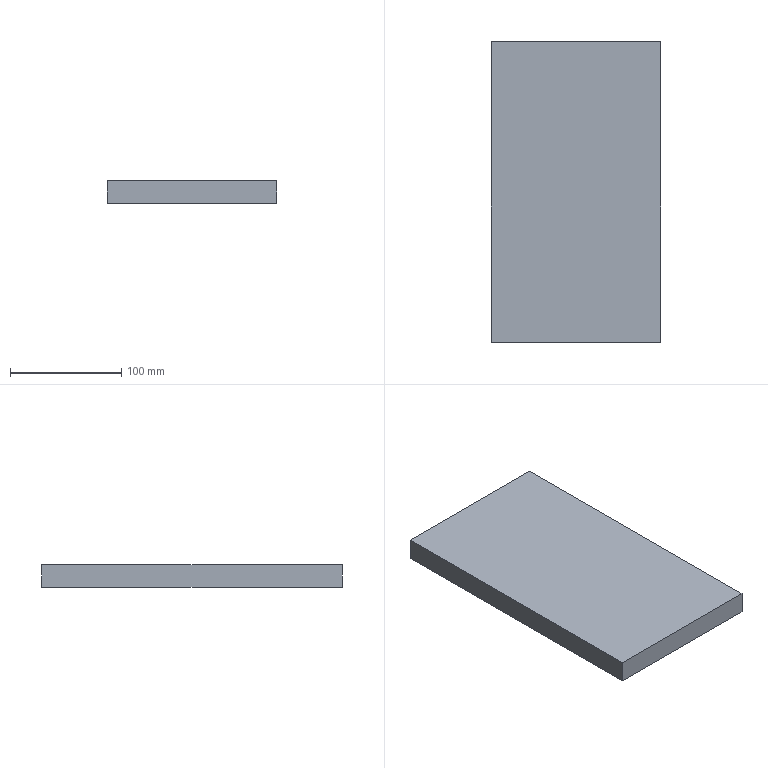Part | SolidWorks | features Extrusion 1 | 1 solid | 6 faces | box 152 x 270 x 20 mm | volume 820800 mm3 | plane 6
STEP:
#1=CARTESIAN_POINT('',(0.,270.,0.));
#2=VERTEX_POINT('',#1);
#3=CARTESIAN_POINT('',(0.,0.,0.));
#4=VERTEX_POINT('',#3);
#5=CARTESIAN_POINT('',(0.,0.,0.));
#6=DIRECTION('',(0.,-1.,0.));
#7=VECTOR('',#6,1000.);
#8=LINE('',#5,#7);
#9=EDGE_CURVE('',#2,#4,#8,.T.);
#10=ORIENTED_EDGE('',*,*,#9,.T.);
#11=CARTESIAN_POINT('',(0.,0.,20.));
#12=VERTEX_POINT('',#11);
#13=CARTESIAN_POINT('',(0.,0.,20.));
#14=DIRECTION('',(0.,0.,-1.));
#15=VECTOR('',#14,1000.);
#16=LINE('',#13,#15);
#17=EDGE_CURVE('',#12,#4,#16,.T.);
#18=ORIENTED_EDGE('',*,*,#17,.F.);
#19=CARTESIAN_POINT('',(0.,270.,20.));
#20=VERTEX_POINT('',#19);
#21=CARTESIAN_POINT('',(0.,0.,20.));
#22=DIRECTION('',(0.,-1.,0.));
#23=VECTOR('',#22,1000.);
#24=LINE('',#21,#23);
#25=EDGE_CURVE('',#20,#12,#24,.T.);
#26=ORIENTED_EDGE('',*,*,#25,.F.);
#27=CARTESIAN_POINT('',(0.,270.,20.));
#28=DIRECTION('',(0.,0.,-1.));
#29=VECTOR('',#28,1000.);
#30=LINE('',#27,#29);
#31=EDGE_CURVE('',#20,#2,#30,.T.);
#32=ORIENTED_EDGE('',*,*,#31,.T.);
#33=EDGE_LOOP('',(#10,#18,#26,#32));
#34=FACE_OUTER_BOUND('',#33,.T.);
#35=CARTESIAN_POINT('',(0.,0.,20.));
#36=DIRECTION('',(1.,0.,0.));
#37=DIRECTION('',(0.,0.,-1.));
#38=AXIS2_PLACEMENT_3D('',#35,#36,#37);
#39=PLANE('',#38);
#40=ADVANCED_FACE('',(#34),#39,.F.);
#41=CARTESIAN_POINT('',(152.,0.,0.));
#42=VERTEX_POINT('',#41);
#43=CARTESIAN_POINT('',(0.,0.,0.));
#44=DIRECTION('',(1.,0.,0.));
#45=VECTOR('',#44,1000.);
#46=LINE('',#43,#45);
#47=EDGE_CURVE('',#4,#42,#46,.T.);
#48=ORIENTED_EDGE('',*,*,#47,.T.);
#49=CARTESIAN_POINT('',(152.,0.,20.));
#50=VERTEX_POINT('',#49);
#51=CARTESIAN_POINT('',(152.,0.,20.));
#52=DIRECTION('',(0.,0.,-1.));
#53=VECTOR('',#52,1000.);
#54=LINE('',#51,#53);
#55=EDGE_CURVE('',#50,#42,#54,.T.);
#56=ORIENTED_EDGE('',*,*,#55,.F.);
#57=CARTESIAN_POINT('',(0.,0.,20.));
#58=DIRECTION('',(1.,0.,0.));
#59=VECTOR('',#58,1000.);
#60=LINE('',#57,#59);
#61=EDGE_CURVE('',#12,#50,#60,.T.);
#62=ORIENTED_EDGE('',*,*,#61,.F.);
#63=ORIENTED_EDGE('',*,*,#17,.T.);
#64=EDGE_LOOP('',(#48,#56,#62,#63));
#65=FACE_OUTER_BOUND('',#64,.T.);
#66=CARTESIAN_POINT('',(0.,0.,20.));
#67=DIRECTION('',(0.,1.,0.));
#68=DIRECTION('',(0.,0.,1.));
#69=AXIS2_PLACEMENT_3D('',#66,#67,#68);
#70=PLANE('',#69);
#71=ADVANCED_FACE('',(#65),#70,.F.);
#72=CARTESIAN_POINT('',(152.,270.,0.));
#73=VERTEX_POINT('',#72);
#74=CARTESIAN_POINT('',(152.,0.,0.));
#75=DIRECTION('',(0.,1.,0.));
#76=VECTOR('',#75,1000.);
#77=LINE('',#74,#76);
#78=EDGE_CURVE('',#42,#73,#77,.T.);
#79=ORIENTED_EDGE('',*,*,#78,.T.);
#80=CARTESIAN_POINT('',(152.,270.,20.));
#81=VERTEX_POINT('',#80);
#82=CARTESIAN_POINT('',(152.,270.,20.));
#83=DIRECTION('',(0.,0.,-1.));
#84=VECTOR('',#83,1000.);
#85=LINE('',#82,#84);
#86=EDGE_CURVE('',#81,#73,#85,.T.);
#87=ORIENTED_EDGE('',*,*,#86,.F.);
#88=CARTESIAN_POINT('',(152.,0.,20.));
#89=DIRECTION('',(0.,1.,0.));
#90=VECTOR('',#89,1000.);
#91=LINE('',#88,#90);
#92=EDGE_CURVE('',#50,#81,#91,.T.);
#93=ORIENTED_EDGE('',*,*,#92,.F.);
#94=ORIENTED_EDGE('',*,*,#55,.T.);
#95=EDGE_LOOP('',(#79,#87,#93,#94));
#96=FACE_OUTER_BOUND('',#95,.T.);
#97=CARTESIAN_POINT('',(152.,0.,20.));
#98=DIRECTION('',(-1.,0.,0.));
#99=DIRECTION('',(0.,0.,1.));
#100=AXIS2_PLACEMENT_3D('',#97,#98,#99);
#101=PLANE('',#100);
#102=ADVANCED_FACE('',(#96),#101,.F.);
#103=CARTESIAN_POINT('',(0.,270.,0.));
#104=DIRECTION('',(-1.,0.,0.));
#105=VECTOR('',#104,1000.);
#106=LINE('',#103,#105);
#107=EDGE_CURVE('',#73,#2,#106,.T.);
#108=ORIENTED_EDGE('',*,*,#107,.T.);
#109=ORIENTED_EDGE('',*,*,#31,.F.);
#110=CARTESIAN_POINT('',(0.,270.,20.));
#111=DIRECTION('',(-1.,0.,0.));
#112=VECTOR('',#111,1000.);
#113=LINE('',#110,#112);
#114=EDGE_CURVE('',#81,#20,#113,.T.);
#115=ORIENTED_EDGE('',*,*,#114,.F.);
#116=ORIENTED_EDGE('',*,*,#86,.T.);
#117=EDGE_LOOP('',(#108,#109,#115,#116));
#118=FACE_OUTER_BOUND('',#117,.T.);
#119=CARTESIAN_POINT('',(0.,270.,20.));
#120=DIRECTION('',(0.,-1.,0.));
#121=DIRECTION('',(0.,0.,-1.));
#122=AXIS2_PLACEMENT_3D('',#119,#120,#121);
#123=PLANE('',#122);
#124=ADVANCED_FACE('',(#118),#123,.F.);
#125=ORIENTED_EDGE('',*,*,#25,.T.);
#126=ORIENTED_EDGE('',*,*,#61,.T.);
#127=ORIENTED_EDGE('',*,*,#92,.T.);
#128=ORIENTED_EDGE('',*,*,#114,.T.);
#129=EDGE_LOOP('',(#125,#126,#127,#128));
#130=FACE_OUTER_BOUND('',#129,.T.);
#131=CARTESIAN_POINT('',(0.,0.,20.));
#132=DIRECTION('',(0.,0.,-1.));
#133=DIRECTION('',(-1.,0.,0.));
#134=AXIS2_PLACEMENT_3D('',#131,#132,#133);
#135=PLANE('',#134);
#136=ADVANCED_FACE('',(#130),#135,.F.);
#137=ORIENTED_EDGE('',*,*,#9,.F.);
#138=ORIENTED_EDGE('',*,*,#107,.F.);
#139=ORIENTED_EDGE('',*,*,#78,.F.);
#140=ORIENTED_EDGE('',*,*,#47,.F.);
#141=EDGE_LOOP('',(#137,#138,#139,#140));
#142=FACE_OUTER_BOUND('',#141,.T.);
#143=CARTESIAN_POINT('',(0.,0.,0.));
#144=DIRECTION('',(0.,0.,-1.));
#145=DIRECTION('',(-1.,0.,0.));
#146=AXIS2_PLACEMENT_3D('',#143,#144,#145);
#147=PLANE('',#146);
#148=ADVANCED_FACE('',(#142),#147,.T.);
#149=CLOSED_SHELL('',(#40,#71,#102,#124,#136,#148));
#150=MANIFOLD_SOLID_BREP('',#149);
#151=CARTESIAN_POINT('',(0.,0.,0.));
#152=DIRECTION('',(0.,0.,1.));
#153=DIRECTION('',(1.,0.,0.));
#154=AXIS2_PLACEMENT_3D('',#151,#152,#153);
#155=(LENGTH_UNIT()NAMED_UNIT(*)SI_UNIT(.MILLI.,.METRE.));
#156=UNCERTAINTY_MEASURE_WITH_UNIT(LENGTH_MEASURE(0.00001),#155,'','');
#157=(NAMED_UNIT(*)PLANE_ANGLE_UNIT()SI_UNIT($,.RADIAN.));
#158=(NAMED_UNIT(*)SI_UNIT($,.STERADIAN.)SOLID_ANGLE_UNIT());
#159=(GEOMETRIC_REPRESENTATION_CONTEXT(3)GLOBAL_UNCERTAINTY_ASSIGNED_CONTEXT((#156))GLOBAL_UNIT_ASSIGNED_CONTEXT((#155,#157,#158))REPRESENTATION_CONTEXT('',''));
#160=ADVANCED_BREP_SHAPE_REPRESENTATION('',(#150,#154),#159);